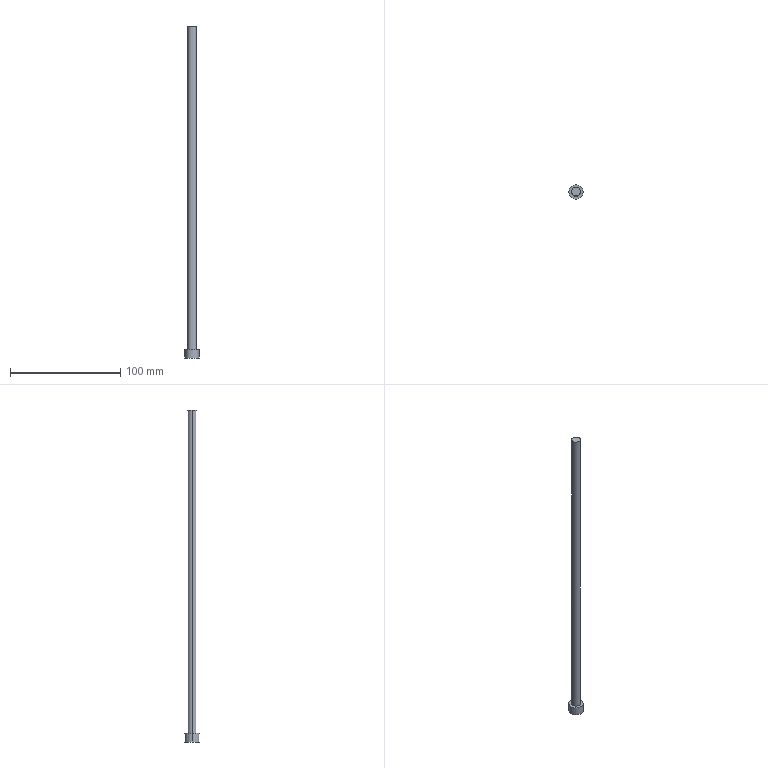Part | Creo | 1 solid | 7 faces | box 13 x 13 x 300.905 mm | volume 15785 mm3 | cylinder 4 | plane 3 | commonest cylinder face diameters 8 x2 13 x2
STEP:
#1=CARTESIAN_POINT('',(-6.089,155.289,40.406));
#2=VERTEX_POINT('',#1);
#3=CARTESIAN_POINT('',(-14.089,155.289,40.406));
#4=VERTEX_POINT('',#3);
#5=CARTESIAN_POINT('',(-10.089,155.289,40.406));
#6=DIRECTION('',(0.,0.,1.));
#7=DIRECTION('',(1.,0.,0.));
#8=AXIS2_PLACEMENT_3D('',#5,#6,#7);
#9=CIRCLE('',#8,4.);
#10=EDGE_CURVE('',#2,#4,#9,.T.);
#11=ORIENTED_EDGE('',*,*,#10,.F.);
#12=CARTESIAN_POINT('',(-10.089,155.289,40.406));
#13=DIRECTION('',(0.,0.,1.));
#14=DIRECTION('',(-1.,0.,0.));
#15=AXIS2_PLACEMENT_3D('',#12,#13,#14);
#16=CIRCLE('',#15,4.);
#17=EDGE_CURVE('',#4,#2,#16,.T.);
#18=ORIENTED_EDGE('',*,*,#17,.F.);
#19=EDGE_LOOP('',(#11,#18));
#20=FACE_OUTER_BOUND('',#19,.F.);
#21=CARTESIAN_POINT('',(-10.089,155.289,40.406));
#22=DIRECTION('',(0.,0.,1.));
#23=DIRECTION('',(1.,0.,0.));
#24=AXIS2_PLACEMENT_3D('',#21,#22,#23);
#25=PLANE('',#24);
#26=ADVANCED_FACE('',(#20),#25,.T.);
#27=CARTESIAN_POINT('',(-14.089,155.289,-252.499));
#28=VERTEX_POINT('',#27);
#29=CARTESIAN_POINT('',(-6.089,155.289,-252.499));
#30=VERTEX_POINT('',#29);
#31=CARTESIAN_POINT('',(-10.089,155.289,-252.499));
#32=DIRECTION('',(0.,0.,-1.));
#33=DIRECTION('',(-1.,0.,0.));
#34=AXIS2_PLACEMENT_3D('',#31,#32,#33);
#35=CIRCLE('',#34,4.);
#36=EDGE_CURVE('',#28,#30,#35,.T.);
#37=ORIENTED_EDGE('',*,*,#36,.T.);
#38=CARTESIAN_POINT('',(-6.089,155.289,-252.499));
#39=DIRECTION('',(0.,0.,1.));
#40=VECTOR('',#39,292.905);
#41=LINE('',#38,#40);
#42=EDGE_CURVE('',#30,#2,#41,.T.);
#43=ORIENTED_EDGE('',*,*,#42,.T.);
#44=ORIENTED_EDGE('',*,*,#10,.T.);
#45=CARTESIAN_POINT('',(-14.089,155.289,-252.499));
#46=DIRECTION('',(0.,0.,1.));
#47=VECTOR('',#46,292.905);
#48=LINE('',#45,#47);
#49=EDGE_CURVE('',#28,#4,#48,.T.);
#50=ORIENTED_EDGE('',*,*,#49,.F.);
#51=EDGE_LOOP('',(#37,#43,#44,#50));
#52=FACE_OUTER_BOUND('',#51,.F.);
#53=CARTESIAN_POINT('',(-10.089,155.289,-255.499));
#54=DIRECTION('',(0.,0.,1.));
#55=DIRECTION('',(1.,0.,0.));
#56=AXIS2_PLACEMENT_3D('',#53,#54,#55);
#57=CYLINDRICAL_SURFACE('',#56,4.);
#58=ADVANCED_FACE('',(#52),#57,.T.);
#59=CARTESIAN_POINT('',(-16.589,155.289,-252.499));
#60=VERTEX_POINT('',#59);
#61=CARTESIAN_POINT('',(-3.589,155.289,-252.499));
#62=VERTEX_POINT('',#61);
#63=CARTESIAN_POINT('',(-10.089,155.289,-252.499));
#64=DIRECTION('',(0.,0.,1.));
#65=DIRECTION('',(-1.,0.,0.));
#66=AXIS2_PLACEMENT_3D('',#63,#64,#65);
#67=CIRCLE('',#66,6.5);
#68=EDGE_CURVE('',#60,#62,#67,.T.);
#69=ORIENTED_EDGE('',*,*,#68,.F.);
#70=CARTESIAN_POINT('',(-10.089,155.289,-252.499));
#71=DIRECTION('',(0.,0.,1.));
#72=DIRECTION('',(1.,0.,0.));
#73=AXIS2_PLACEMENT_3D('',#70,#71,#72);
#74=CIRCLE('',#73,6.5);
#75=EDGE_CURVE('',#62,#60,#74,.T.);
#76=ORIENTED_EDGE('',*,*,#75,.F.);
#77=EDGE_LOOP('',(#69,#76));
#78=FACE_OUTER_BOUND('',#77,.F.);
#79=CARTESIAN_POINT('',(-10.089,155.289,-252.499));
#80=DIRECTION('',(0.,0.,-1.));
#81=DIRECTION('',(1.,0.,0.));
#82=AXIS2_PLACEMENT_3D('',#79,#80,#81);
#83=CIRCLE('',#82,4.);
#84=EDGE_CURVE('',#30,#28,#83,.T.);
#85=ORIENTED_EDGE('',*,*,#84,.F.);
#86=ORIENTED_EDGE('',*,*,#36,.F.);
#87=EDGE_LOOP('',(#85,#86));
#88=FACE_BOUND('',#87,.F.);
#89=CARTESIAN_POINT('',(-10.089,155.289,-252.499));
#90=DIRECTION('',(0.,0.,1.));
#91=DIRECTION('',(1.,0.,0.));
#92=AXIS2_PLACEMENT_3D('',#89,#90,#91);
#93=PLANE('',#92);
#94=ADVANCED_FACE('',(#78,#88),#93,.T.);
#95=ORIENTED_EDGE('',*,*,#84,.T.);
#96=ORIENTED_EDGE('',*,*,#49,.T.);
#97=ORIENTED_EDGE('',*,*,#17,.T.);
#98=ORIENTED_EDGE('',*,*,#42,.F.);
#99=EDGE_LOOP('',(#95,#96,#97,#98));
#100=FACE_OUTER_BOUND('',#99,.F.);
#101=CARTESIAN_POINT('',(-10.089,155.289,-255.499));
#102=DIRECTION('',(0.,0.,1.));
#103=DIRECTION('',(1.,0.,0.));
#104=AXIS2_PLACEMENT_3D('',#101,#102,#103);
#105=CYLINDRICAL_SURFACE('',#104,4.);
#106=ADVANCED_FACE('',(#100),#105,.T.);
#107=ORIENTED_EDGE('',*,*,#68,.T.);
#108=CARTESIAN_POINT('',(-3.589,155.289,-260.499));
#109=VERTEX_POINT('',#108);
#110=CARTESIAN_POINT('',(-3.589,155.289,-260.499));
#111=DIRECTION('',(0.,0.,1.));
#112=VECTOR('',#111,8.);
#113=LINE('',#110,#112);
#114=EDGE_CURVE('',#109,#62,#113,.T.);
#115=ORIENTED_EDGE('',*,*,#114,.F.);
#116=CARTESIAN_POINT('',(-16.589,155.289,-260.499));
#117=VERTEX_POINT('',#116);
#118=CARTESIAN_POINT('',(-10.089,155.289,-260.499));
#119=DIRECTION('',(0.,0.,-1.));
#120=DIRECTION('',(1.,0.,0.));
#121=AXIS2_PLACEMENT_3D('',#118,#119,#120);
#122=CIRCLE('',#121,6.5);
#123=EDGE_CURVE('',#109,#117,#122,.T.);
#124=ORIENTED_EDGE('',*,*,#123,.T.);
#125=CARTESIAN_POINT('',(-16.589,155.289,-260.499));
#126=DIRECTION('',(0.,0.,1.));
#127=VECTOR('',#126,8.);
#128=LINE('',#125,#127);
#129=EDGE_CURVE('',#117,#60,#128,.T.);
#130=ORIENTED_EDGE('',*,*,#129,.T.);
#131=EDGE_LOOP('',(#107,#115,#124,#130));
#132=FACE_OUTER_BOUND('',#131,.F.);
#133=CARTESIAN_POINT('',(-10.089,155.289,-260.499));
#134=DIRECTION('',(0.,0.,1.));
#135=DIRECTION('',(1.,0.,0.));
#136=AXIS2_PLACEMENT_3D('',#133,#134,#135);
#137=CYLINDRICAL_SURFACE('',#136,6.5);
#138=ADVANCED_FACE('',(#132),#137,.T.);
#139=ORIENTED_EDGE('',*,*,#75,.T.);
#140=ORIENTED_EDGE('',*,*,#129,.F.);
#141=CARTESIAN_POINT('',(-10.089,155.289,-260.499));
#142=DIRECTION('',(0.,0.,-1.));
#143=DIRECTION('',(-1.,0.,0.));
#144=AXIS2_PLACEMENT_3D('',#141,#142,#143);
#145=CIRCLE('',#144,6.5);
#146=EDGE_CURVE('',#117,#109,#145,.T.);
#147=ORIENTED_EDGE('',*,*,#146,.T.);
#148=ORIENTED_EDGE('',*,*,#114,.T.);
#149=EDGE_LOOP('',(#139,#140,#147,#148));
#150=FACE_OUTER_BOUND('',#149,.F.);
#151=CARTESIAN_POINT('',(-10.089,155.289,-260.499));
#152=DIRECTION('',(0.,0.,1.));
#153=DIRECTION('',(1.,0.,0.));
#154=AXIS2_PLACEMENT_3D('',#151,#152,#153);
#155=CYLINDRICAL_SURFACE('',#154,6.5);
#156=ADVANCED_FACE('',(#150),#155,.T.);
#157=ORIENTED_EDGE('',*,*,#123,.F.);
#158=ORIENTED_EDGE('',*,*,#146,.F.);
#159=EDGE_LOOP('',(#157,#158));
#160=FACE_OUTER_BOUND('',#159,.F.);
#161=CARTESIAN_POINT('',(-10.089,155.289,-260.499));
#162=DIRECTION('',(0.,0.,-1.));
#163=DIRECTION('',(-1.,0.,0.));
#164=AXIS2_PLACEMENT_3D('',#161,#162,#163);
#165=PLANE('',#164);
#166=ADVANCED_FACE('',(#160),#165,.T.);
#167=CLOSED_SHELL('',(#26,#58,#94,#106,#138,#156,#166));
#168=MANIFOLD_SOLID_BREP('',#167);
#169=(LENGTH_UNIT()NAMED_UNIT(*)SI_UNIT(.MILLI.,.METRE.));
#170=UNCERTAINTY_MEASURE_WITH_UNIT(LENGTH_MEASURE(0.03015),#169,'','');
#171=(NAMED_UNIT(*)PLANE_ANGLE_UNIT()SI_UNIT($,.RADIAN.));
#172=PLANE_ANGLE_MEASURE_WITH_UNIT(PLANE_ANGLE_MEASURE(0.01745),#171);
#173=(CONVERSION_BASED_UNIT('DEGREE',#172)NAMED_UNIT(*)PLANE_ANGLE_UNIT());
#174=(NAMED_UNIT(*)SI_UNIT($,.STERADIAN.)SOLID_ANGLE_UNIT());
#175=(GEOMETRIC_REPRESENTATION_CONTEXT(3)GLOBAL_UNCERTAINTY_ASSIGNED_CONTEXT((#170))GLOBAL_UNIT_ASSIGNED_CONTEXT((#169,#173,#174))REPRESENTATION_CONTEXT('',''));
#176=ADVANCED_BREP_SHAPE_REPRESENTATION('',(#168),#175);